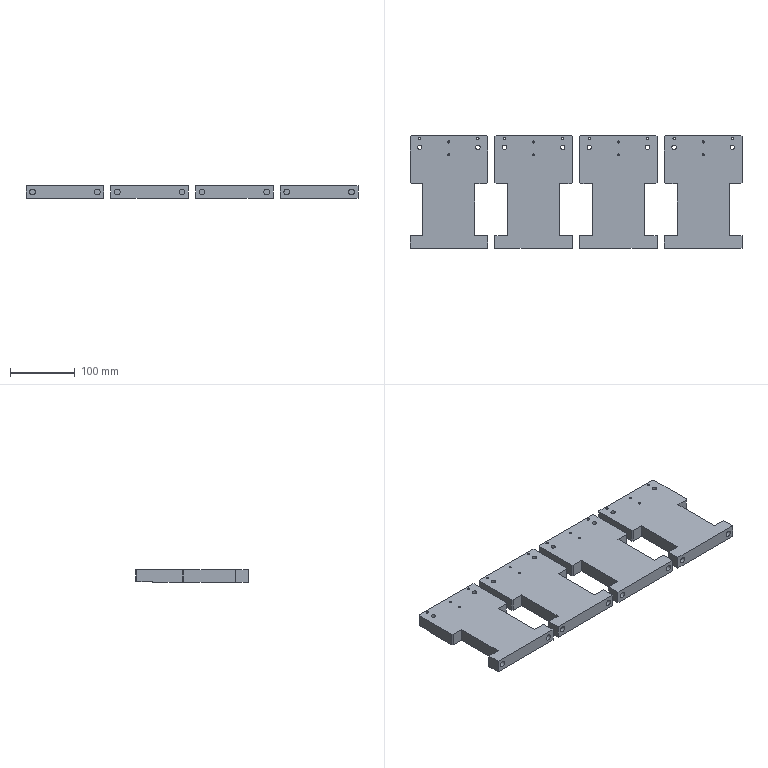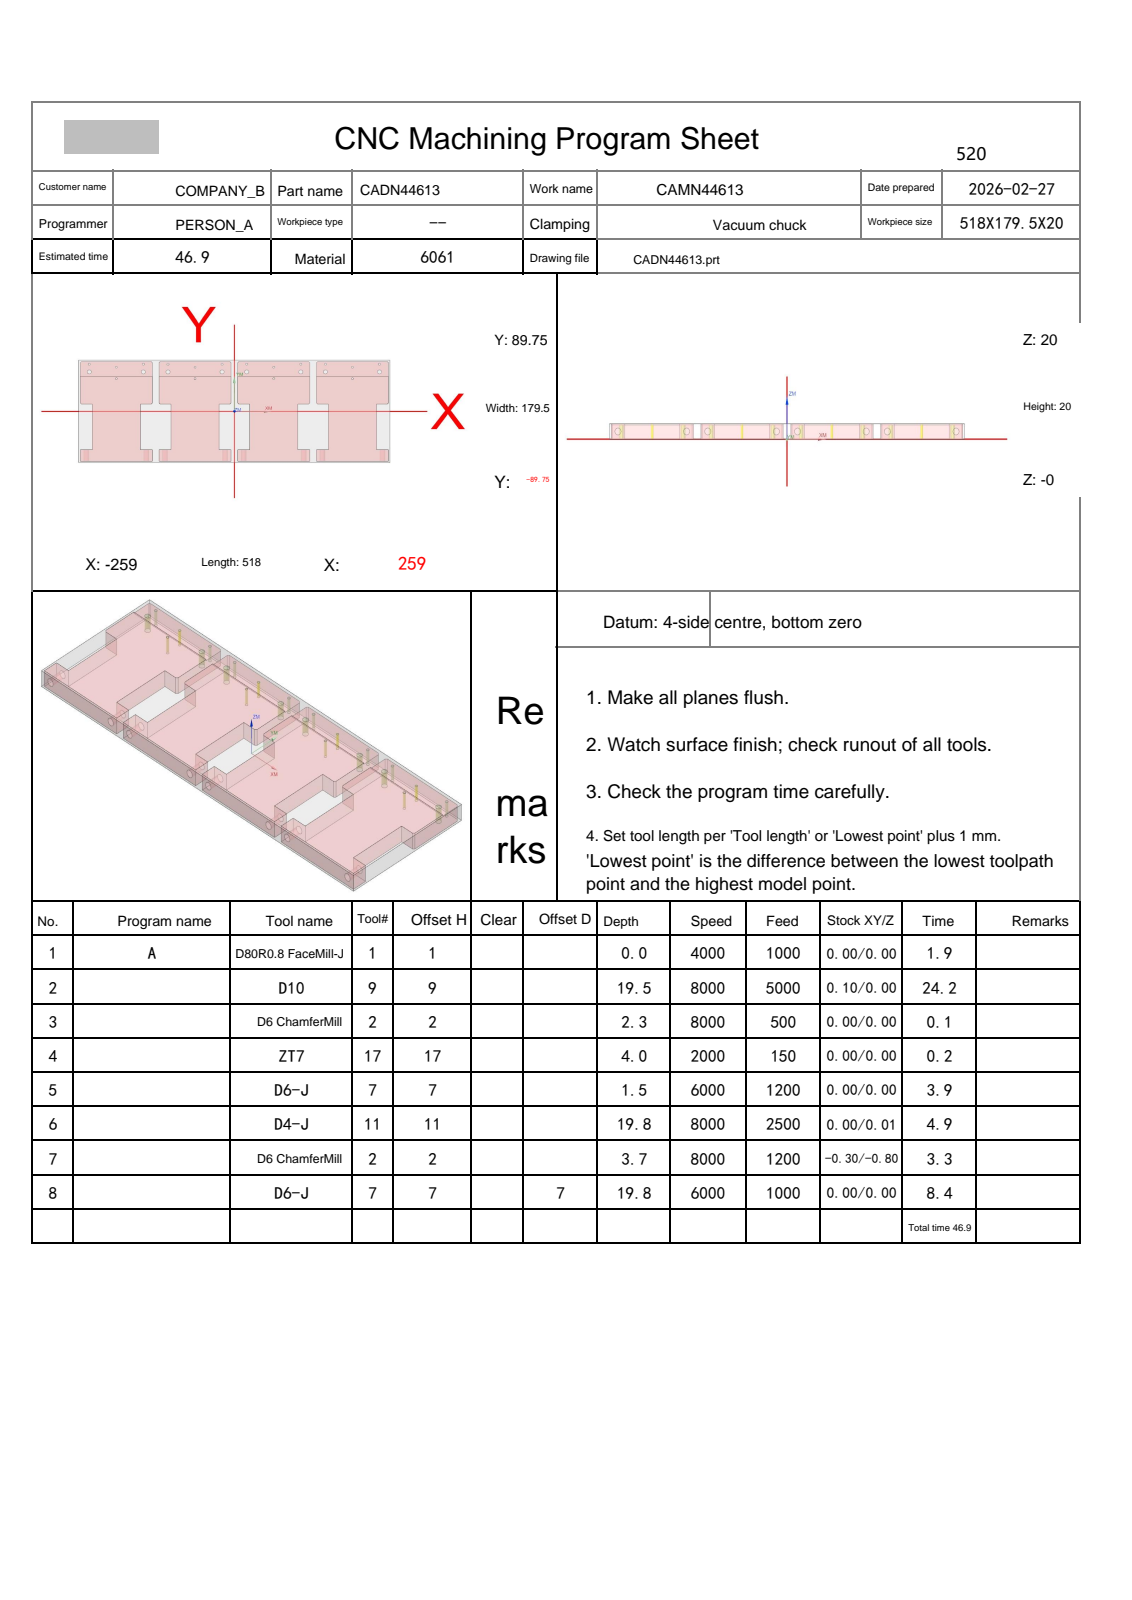NC program | NX | posted by the shop | part box 513 x 174.5 x 20 mm
Lines 5165 to 6116 of 36838:
N6 T11 M06
(D4-J  D=4. R=0. H=11 ce=0.00 di=0.01)
G00 G90 G54 X-242.053 Y-64.649 M03 S8000
G43 H11 Z50.
M08
Z20.3
G01 X-242.052 Y-64.655 Z20.214 F2000.
X-242.049 Y-64.675 Z20.136
X-242.044 Y-64.704 Z20.066
X-242.036 Y-64.743 Z20.004
X-242.025 Y-64.788 Z19.948
X-242.011 Y-64.839 Z19.899
X-241.994 Y-64.893 Z19.857
X-241.973 Y-64.949 Z19.82
X-241.949 Y-65.005 Z19.789
X-241.92 Y-65.06 Z19.763
X-241.888 Y-65.111 Z19.742
X-241.851 Y-65.156 Z19.726
X-241.809 Y-65.195 Z19.714
X-241.762 Y-65.224 Z19.706
X-241.71 Y-65.243 Z19.701
X-241.653 Y-65.25 Z19.7
X-238.5 F2500.
Y-62.097
X-238.516 Y-62.054 Z19.699
X-238.562 Y-62.032 Z19.696
X-238.634 Y-62.031 Z19.692
X-238.729 Y-62.048 Z19.687
X-238.844 Y-62.081 Z19.68
X-238.974 Y-62.13 Z19.672
X-239.118 Y-62.193 Z19.662
X-239.27 Y-62.267 Z19.653
X-239.429 Y-62.352 Z19.642
X-239.59 Y-62.446 Z19.631
X-239.75 Y-62.546 Z19.619
X-240.087 Y-62.788 Z19.592
X-240.403 Y-63.055 Z19.564
X-240.694 Y-63.347 Z19.536
X-240.962 Y-63.662 Z19.508
X-241.203 Y-64. Z19.481
X-241.304 Y-64.16 Z19.469
X-241.398 Y-64.321 Z19.458
X-241.483 Y-64.479 Z19.447
X-241.557 Y-64.632 Z19.438
X-241.62 Y-64.775 Z19.428
X-241.669 Y-64.906 Z19.42
X-241.702 Y-65.021 Z19.413
X-241.719 Y-65.116 Z19.408
X-241.718 Y-65.188 Z19.404
X-241.696 Y-65.234 Z19.401
X-241.653 Y-65.25 Z19.4
X-238.5
Y-62.097
X-238.516 Y-62.054 Z19.399
X-238.562 Y-62.032 Z19.396
X-238.634 Y-62.031 Z19.392
X-238.729 Y-62.048 Z19.387
X-238.844 Y-62.081 Z19.38
X-238.974 Y-62.13 Z19.372
X-239.118 Y-62.193 Z19.362
X-239.27 Y-62.267 Z19.353
X-239.429 Y-62.352 Z19.342
X-239.59 Y-62.446 Z19.331
X-239.75 Y-62.546 Z19.319
X-240.087 Y-62.788 Z19.292
X-240.403 Y-63.055 Z19.264
X-240.694 Y-63.347 Z19.236
X-240.962 Y-63.662 Z19.208
X-241.203 Y-64. Z19.181
X-241.304 Y-64.16 Z19.169
X-241.398 Y-64.321 Z19.158
X-241.483 Y-64.479 Z19.147
X-241.557 Y-64.632 Z19.138
X-241.62 Y-64.775 Z19.128
X-241.669 Y-64.906 Z19.12
X-241.702 Y-65.021 Z19.113
X-241.719 Y-65.116 Z19.108
X-241.718 Y-65.188 Z19.104
X-241.696 Y-65.234 Z19.101
X-241.653 Y-65.25 Z19.1
X-238.5
Y-62.097
X-238.516 Y-62.054 Z19.099
X-238.562 Y-62.032 Z19.096
X-238.634 Y-62.031 Z19.092
X-238.729 Y-62.048 Z19.087
X-238.844 Y-62.081 Z19.08
X-238.974 Y-62.13 Z19.072
X-239.118 Y-62.193 Z19.062
X-239.27 Y-62.267 Z19.053
X-239.429 Y-62.352 Z19.042
X-239.59 Y-62.446 Z19.031
X-239.75 Y-62.546 Z19.019
X-240.087 Y-62.788 Z18.992
X-240.403 Y-63.055 Z18.964
X-240.694 Y-63.347 Z18.936
X-240.962 Y-63.662 Z18.908
X-241.203 Y-64. Z18.881
X-241.304 Y-64.16 Z18.869
X-241.398 Y-64.321 Z18.858
X-241.483 Y-64.479 Z18.847
X-241.557 Y-64.632 Z18.838
X-241.62 Y-64.775 Z18.828
X-241.669 Y-64.906 Z18.82
X-241.702 Y-65.021 Z18.813
X-241.719 Y-65.116 Z18.808
X-241.718 Y-65.188 Z18.804
X-241.696 Y-65.234 Z18.801
X-241.653 Y-65.25 Z18.8
X-238.5
Y-62.097
X-238.516 Y-62.054 Z18.799
X-238.562 Y-62.032 Z18.796
X-238.634 Y-62.031 Z18.792
X-238.729 Y-62.048 Z18.787
X-238.844 Y-62.081 Z18.78
X-238.974 Y-62.13 Z18.772
X-239.118 Y-62.193 Z18.762
X-239.27 Y-62.267 Z18.753
X-239.429 Y-62.352 Z18.742
X-239.59 Y-62.446 Z18.731
X-239.75 Y-62.546 Z18.719
X-240.087 Y-62.788 Z18.692
X-240.403 Y-63.055 Z18.664
X-240.694 Y-63.347 Z18.636
X-240.962 Y-63.662 Z18.608
X-241.203 Y-64. Z18.581
X-241.304 Y-64.16 Z18.569
X-241.398 Y-64.321 Z18.558
X-241.483 Y-64.479 Z18.547
X-241.557 Y-64.632 Z18.538
X-241.62 Y-64.775 Z18.528
X-241.669 Y-64.906 Z18.52
X-241.702 Y-65.021 Z18.513
X-241.719 Y-65.116 Z18.508
X-241.718 Y-65.188 Z18.504
X-241.696 Y-65.234 Z18.501
X-241.653 Y-65.25 Z18.5
X-238.5
Y-62.097
X-238.516 Y-62.054 Z18.499
X-238.562 Y-62.032 Z18.496
X-238.634 Y-62.031 Z18.492
X-238.729 Y-62.048 Z18.487
X-238.844 Y-62.081 Z18.48
X-238.974 Y-62.13 Z18.472
X-239.118 Y-62.193 Z18.462
X-239.27 Y-62.267 Z18.453
X-239.429 Y-62.352 Z18.442
X-239.59 Y-62.446 Z18.431
X-239.75 Y-62.546 Z18.419
X-240.087 Y-62.788 Z18.392
X-240.403 Y-63.055 Z18.364
X-240.694 Y-63.347 Z18.336
X-240.962 Y-63.662 Z18.308
X-241.203 Y-64. Z18.281
X-241.304 Y-64.16 Z18.269
X-241.398 Y-64.321 Z18.258
X-241.483 Y-64.479 Z18.247
X-241.557 Y-64.632 Z18.238
X-241.62 Y-64.775 Z18.228
X-241.669 Y-64.906 Z18.22
X-241.702 Y-65.021 Z18.213
X-241.719 Y-65.116 Z18.208
X-241.718 Y-65.188 Z18.204
X-241.696 Y-65.234 Z18.201
X-241.653 Y-65.25 Z18.2
X-238.5
Y-62.097
X-238.516 Y-62.054 Z18.199
X-238.562 Y-62.032 Z18.196
X-238.634 Y-62.031 Z18.192
X-238.729 Y-62.048 Z18.187
X-238.844 Y-62.081 Z18.18
X-238.974 Y-62.13 Z18.172
X-239.118 Y-62.193 Z18.162
X-239.27 Y-62.267 Z18.153
X-239.429 Y-62.352 Z18.142
X-239.59 Y-62.446 Z18.131
X-239.75 Y-62.546 Z18.119
X-240.087 Y-62.788 Z18.092
X-240.403 Y-63.055 Z18.064
X-240.694 Y-63.347 Z18.036
X-240.962 Y-63.662 Z18.008
X-241.203 Y-64. Z17.981
X-241.304 Y-64.16 Z17.969
X-241.398 Y-64.321 Z17.958
X-241.483 Y-64.479 Z17.947
X-241.557 Y-64.632 Z17.938
X-241.62 Y-64.775 Z17.928
X-241.669 Y-64.906 Z17.92
X-241.702 Y-65.021 Z17.913
X-241.719 Y-65.116 Z17.908
X-241.718 Y-65.188 Z17.904
X-241.696 Y-65.234 Z17.901
X-241.653 Y-65.25 Z17.9
X-238.5
Y-62.097
X-238.516 Y-62.054 Z17.899
X-238.562 Y-62.032 Z17.896
X-238.634 Y-62.031 Z17.892
X-238.729 Y-62.048 Z17.887
X-238.844 Y-62.081 Z17.88
X-238.974 Y-62.13 Z17.872
X-239.118 Y-62.193 Z17.862
X-239.27 Y-62.267 Z17.853
X-239.429 Y-62.352 Z17.842
X-239.59 Y-62.446 Z17.831
X-239.75 Y-62.546 Z17.819
X-240.087 Y-62.788 Z17.792
X-240.403 Y-63.055 Z17.764
X-240.694 Y-63.347 Z17.736
X-240.962 Y-63.662 Z17.708
X-241.203 Y-64. Z17.681
X-241.304 Y-64.16 Z17.669
X-241.398 Y-64.321 Z17.658
X-241.483 Y-64.479 Z17.647
X-241.557 Y-64.632 Z17.638
X-241.62 Y-64.775 Z17.628
X-241.669 Y-64.906 Z17.62
X-241.702 Y-65.021 Z17.613
X-241.719 Y-65.116 Z17.608
X-241.718 Y-65.188 Z17.604
X-241.696 Y-65.234 Z17.601
X-241.653 Y-65.25 Z17.6
X-238.5
Y-62.097
X-238.516 Y-62.054 Z17.599
X-238.562 Y-62.032 Z17.596
X-238.634 Y-62.031 Z17.592
X-238.729 Y-62.048 Z17.587
X-238.844 Y-62.081 Z17.58
X-238.974 Y-62.13 Z17.572
X-239.118 Y-62.193 Z17.562
X-239.27 Y-62.267 Z17.553
X-239.429 Y-62.352 Z17.542
X-239.59 Y-62.446 Z17.531
X-239.75 Y-62.546 Z17.519
X-240.087 Y-62.788 Z17.492
X-240.403 Y-63.055 Z17.464
X-240.694 Y-63.347 Z17.436
X-240.962 Y-63.662 Z17.408
X-241.203 Y-64. Z17.381
X-241.304 Y-64.16 Z17.369
X-241.398 Y-64.321 Z17.358
X-241.483 Y-64.479 Z17.347
X-241.557 Y-64.632 Z17.338
X-241.62 Y-64.775 Z17.328
X-241.669 Y-64.906 Z17.32
X-241.702 Y-65.021 Z17.313
X-241.719 Y-65.116 Z17.308
X-241.718 Y-65.188 Z17.304
X-241.696 Y-65.234 Z17.301
X-241.653 Y-65.25 Z17.3
X-238.5
Y-62.097
X-238.516 Y-62.054 Z17.299
X-238.562 Y-62.032 Z17.296
X-238.634 Y-62.031 Z17.292
X-238.729 Y-62.048 Z17.287
X-238.844 Y-62.081 Z17.28
X-238.974 Y-62.13 Z17.272
X-239.118 Y-62.193 Z17.262
X-239.27 Y-62.267 Z17.253
X-239.429 Y-62.352 Z17.242
X-239.59 Y-62.446 Z17.231
X-239.75 Y-62.546 Z17.219
X-240.087 Y-62.788 Z17.192
X-240.403 Y-63.055 Z17.164
X-240.694 Y-63.347 Z17.136
X-240.962 Y-63.662 Z17.108
X-241.203 Y-64. Z17.081
X-241.304 Y-64.16 Z17.069
X-241.398 Y-64.321 Z17.058
X-241.483 Y-64.479 Z17.047
X-241.557 Y-64.632 Z17.038
X-241.62 Y-64.775 Z17.028
X-241.669 Y-64.906 Z17.02
X-241.702 Y-65.021 Z17.013
X-241.719 Y-65.116 Z17.008
X-241.718 Y-65.188 Z17.004
X-241.696 Y-65.234 Z17.001
X-241.653 Y-65.25 Z17.
X-238.5
Y-62.097
X-238.516 Y-62.054 Z16.999
X-238.562 Y-62.032 Z16.996
X-238.634 Y-62.031 Z16.992
X-238.729 Y-62.048 Z16.987
X-238.844 Y-62.081 Z16.98
X-238.974 Y-62.13 Z16.972
X-239.118 Y-62.193 Z16.962
X-239.27 Y-62.267 Z16.953
X-239.429 Y-62.352 Z16.942
X-239.59 Y-62.446 Z16.931
X-239.75 Y-62.546 Z16.919
X-240.087 Y-62.788 Z16.892
X-240.403 Y-63.055 Z16.864
X-240.694 Y-63.347 Z16.836
X-240.962 Y-63.662 Z16.808
X-241.203 Y-64. Z16.781
X-241.304 Y-64.16 Z16.769
X-241.398 Y-64.321 Z16.758
X-241.483 Y-64.479 Z16.747
X-241.557 Y-64.632 Z16.738
X-241.62 Y-64.775 Z16.728
X-241.669 Y-64.906 Z16.72
X-241.702 Y-65.021 Z16.713
X-241.719 Y-65.116 Z16.708
X-241.718 Y-65.188 Z16.704
X-241.696 Y-65.234 Z16.701
X-241.653 Y-65.25 Z16.7
X-238.5
Y-62.097
X-238.516 Y-62.054 Z16.699
X-238.562 Y-62.032 Z16.696
X-238.634 Y-62.031 Z16.692
X-238.729 Y-62.048 Z16.687
X-238.844 Y-62.081 Z16.68
X-238.974 Y-62.13 Z16.672
X-239.118 Y-62.193 Z16.662
X-239.27 Y-62.267 Z16.653
X-239.429 Y-62.352 Z16.642
X-239.59 Y-62.446 Z16.631
X-239.75 Y-62.546 Z16.619
X-240.087 Y-62.788 Z16.592
X-240.403 Y-63.055 Z16.564
X-240.694 Y-63.347 Z16.536
X-240.962 Y-63.662 Z16.508
X-241.203 Y-64. Z16.481
X-241.304 Y-64.16 Z16.469
X-241.398 Y-64.321 Z16.458
X-241.483 Y-64.479 Z16.447
X-241.557 Y-64.632 Z16.438
X-241.62 Y-64.775 Z16.428
X-241.669 Y-64.906 Z16.42
X-241.702 Y-65.021 Z16.413
X-241.719 Y-65.116 Z16.408
X-241.718 Y-65.188 Z16.404
X-241.696 Y-65.234 Z16.401
X-241.653 Y-65.25 Z16.4
X-238.5
Y-62.097
X-238.516 Y-62.054 Z16.399
X-238.562 Y-62.032 Z16.396
X-238.634 Y-62.031 Z16.392
X-238.729 Y-62.048 Z16.387
X-238.844 Y-62.081 Z16.38
X-238.974 Y-62.13 Z16.372
X-239.118 Y-62.193 Z16.362
X-239.27 Y-62.267 Z16.353
X-239.429 Y-62.352 Z16.342
X-239.59 Y-62.446 Z16.331
X-239.75 Y-62.546 Z16.319
X-240.087 Y-62.788 Z16.292
X-240.403 Y-63.055 Z16.264
X-240.694 Y-63.347 Z16.236
X-240.962 Y-63.662 Z16.208
X-241.203 Y-64. Z16.181
X-241.304 Y-64.16 Z16.169
X-241.398 Y-64.321 Z16.158
X-241.483 Y-64.479 Z16.147
X-241.557 Y-64.632 Z16.138
X-241.62 Y-64.775 Z16.128
X-241.669 Y-64.906 Z16.12
X-241.702 Y-65.021 Z16.113
X-241.719 Y-65.116 Z16.108
X-241.718 Y-65.188 Z16.104
X-241.696 Y-65.234 Z16.101
X-241.653 Y-65.25 Z16.1
X-238.5
Y-62.097
X-238.516 Y-62.054 Z16.099
X-238.562 Y-62.032 Z16.096
X-238.634 Y-62.031 Z16.092
X-238.729 Y-62.048 Z16.087
X-238.844 Y-62.081 Z16.08
X-238.974 Y-62.13 Z16.072
X-239.118 Y-62.193 Z16.062
X-239.27 Y-62.267 Z16.053
X-239.429 Y-62.352 Z16.042
X-239.59 Y-62.446 Z16.031
X-239.75 Y-62.546 Z16.019
X-240.087 Y-62.788 Z15.992
X-240.403 Y-63.055 Z15.964
X-240.694 Y-63.347 Z15.936
X-240.962 Y-63.662 Z15.908
X-241.203 Y-64. Z15.881
X-241.304 Y-64.16 Z15.869
X-241.398 Y-64.321 Z15.858
X-241.483 Y-64.479 Z15.847
X-241.557 Y-64.632 Z15.838
X-241.62 Y-64.775 Z15.828
X-241.669 Y-64.906 Z15.82
X-241.702 Y-65.021 Z15.813
X-241.719 Y-65.116 Z15.808
X-241.718 Y-65.188 Z15.804
X-241.696 Y-65.234 Z15.801
X-241.653 Y-65.25 Z15.8
X-238.5
Y-62.097
X-238.516 Y-62.054 Z15.799
X-238.562 Y-62.032 Z15.796
X-238.634 Y-62.031 Z15.792
X-238.729 Y-62.048 Z15.787
X-238.844 Y-62.081 Z15.78
X-238.974 Y-62.13 Z15.772
X-239.118 Y-62.193 Z15.762
X-239.27 Y-62.267 Z15.753
X-239.429 Y-62.352 Z15.742
X-239.59 Y-62.446 Z15.731
X-239.75 Y-62.546 Z15.719
X-240.087 Y-62.788 Z15.692
X-240.403 Y-63.055 Z15.664
X-240.694 Y-63.347 Z15.636
X-240.962 Y-63.662 Z15.608
X-241.203 Y-64. Z15.581
X-241.304 Y-64.16 Z15.569
X-241.398 Y-64.321 Z15.558
X-241.483 Y-64.479 Z15.547
X-241.557 Y-64.632 Z15.538
X-241.62 Y-64.775 Z15.528
X-241.669 Y-64.906 Z15.52
X-241.702 Y-65.021 Z15.513
X-241.719 Y-65.116 Z15.508
X-241.718 Y-65.188 Z15.504
X-241.696 Y-65.234 Z15.501
X-241.653 Y-65.25 Z15.5
X-238.5
Y-62.097
X-238.516 Y-62.054 Z15.499
X-238.562 Y-62.032 Z15.496
X-238.634 Y-62.031 Z15.492
X-238.729 Y-62.048 Z15.487
X-238.844 Y-62.081 Z15.48
X-238.974 Y-62.13 Z15.472
X-239.118 Y-62.193 Z15.462
X-239.27 Y-62.267 Z15.453
X-239.429 Y-62.352 Z15.442
X-239.59 Y-62.446 Z15.431
X-239.75 Y-62.546 Z15.419
X-240.087 Y-62.788 Z15.392
X-240.403 Y-63.055 Z15.364
X-240.694 Y-63.347 Z15.336
X-240.962 Y-63.662 Z15.308
X-241.203 Y-64. Z15.281
X-241.304 Y-64.16 Z15.269
X-241.398 Y-64.321 Z15.258
X-241.483 Y-64.479 Z15.247
X-241.557 Y-64.632 Z15.238
X-241.62 Y-64.775 Z15.228
X-241.669 Y-64.906 Z15.22
X-241.702 Y-65.021 Z15.213
X-241.719 Y-65.116 Z15.208
X-241.718 Y-65.188 Z15.204
X-241.696 Y-65.234 Z15.201
X-241.653 Y-65.25 Z15.2
X-238.5
Y-62.097
X-238.516 Y-62.054 Z15.199
X-238.562 Y-62.032 Z15.196
X-238.634 Y-62.031 Z15.192
X-238.729 Y-62.048 Z15.187
X-238.844 Y-62.081 Z15.18
X-238.974 Y-62.13 Z15.172
X-239.118 Y-62.193 Z15.162
X-239.27 Y-62.267 Z15.153
X-239.429 Y-62.352 Z15.142
X-239.59 Y-62.446 Z15.131
X-239.75 Y-62.546 Z15.119
X-240.087 Y-62.788 Z15.092
X-240.403 Y-63.055 Z15.064
X-240.694 Y-63.347 Z15.036
X-240.962 Y-63.662 Z15.008
X-241.203 Y-64. Z14.981
X-241.304 Y-64.16 Z14.969
X-241.398 Y-64.321 Z14.958
X-241.483 Y-64.479 Z14.947
X-241.557 Y-64.632 Z14.938
X-241.62 Y-64.775 Z14.928
X-241.669 Y-64.906 Z14.92
X-241.702 Y-65.021 Z14.913
X-241.719 Y-65.116 Z14.908
X-241.718 Y-65.188 Z14.904
X-241.696 Y-65.234 Z14.901
X-241.653 Y-65.25 Z14.9
X-238.5
Y-62.097
X-238.516 Y-62.054 Z14.899
X-238.562 Y-62.032 Z14.896
X-238.634 Y-62.031 Z14.892
X-238.729 Y-62.048 Z14.887
X-238.844 Y-62.081 Z14.88
X-238.974 Y-62.13 Z14.872
X-239.118 Y-62.193 Z14.862
X-239.27 Y-62.267 Z14.853
X-239.429 Y-62.352 Z14.842
X-239.59 Y-62.446 Z14.831
X-239.75 Y-62.546 Z14.819
X-240.087 Y-62.788 Z14.792
X-240.403 Y-63.055 Z14.764
X-240.694 Y-63.347 Z14.736
X-240.962 Y-63.662 Z14.708
X-241.203 Y-64. Z14.681
X-241.304 Y-64.16 Z14.669
X-241.398 Y-64.321 Z14.658
X-241.483 Y-64.479 Z14.647
X-241.557 Y-64.632 Z14.638
X-241.62 Y-64.775 Z14.628
X-241.669 Y-64.906 Z14.62
X-241.702 Y-65.021 Z14.613
X-241.719 Y-65.116 Z14.608
X-241.718 Y-65.188 Z14.604
X-241.696 Y-65.234 Z14.601
X-241.653 Y-65.25 Z14.6
X-238.5
Y-62.097
X-238.516 Y-62.054 Z14.599
X-238.562 Y-62.032 Z14.596
X-238.634 Y-62.031 Z14.592
X-238.729 Y-62.048 Z14.587
X-238.844 Y-62.081 Z14.58
X-238.974 Y-62.13 Z14.572
X-239.118 Y-62.193 Z14.562
X-239.27 Y-62.267 Z14.553
X-239.429 Y-62.352 Z14.542
X-239.59 Y-62.446 Z14.531
X-239.75 Y-62.546 Z14.519
X-240.087 Y-62.788 Z14.492
X-240.403 Y-63.055 Z14.464
X-240.694 Y-63.347 Z14.436
X-240.962 Y-63.662 Z14.408
X-241.203 Y-64. Z14.381
X-241.304 Y-64.16 Z14.369
X-241.398 Y-64.321 Z14.358
X-241.483 Y-64.479 Z14.347
X-241.557 Y-64.632 Z14.338
X-241.62 Y-64.775 Z14.328
X-241.669 Y-64.906 Z14.32
X-241.702 Y-65.021 Z14.313
X-241.719 Y-65.116 Z14.308
X-241.718 Y-65.188 Z14.304
X-241.696 Y-65.234 Z14.301
X-241.653 Y-65.25 Z14.3
X-238.5
Y-62.097
X-238.516 Y-62.054 Z14.299
X-238.562 Y-62.032 Z14.296
X-238.634 Y-62.031 Z14.292
X-238.729 Y-62.048 Z14.287
X-238.844 Y-62.081 Z14.28
X-238.974 Y-62.13 Z14.272
X-239.118 Y-62.193 Z14.262
X-239.27 Y-62.267 Z14.253
X-239.429 Y-62.352 Z14.242
X-239.59 Y-62.446 Z14.231
X-239.75 Y-62.546 Z14.219
X-240.087 Y-62.788 Z14.192
X-240.403 Y-63.055 Z14.164
X-240.694 Y-63.347 Z14.136
X-240.962 Y-63.662 Z14.108
X-241.203 Y-64. Z14.081
X-241.304 Y-64.16 Z14.069
X-241.398 Y-64.321 Z14.058
X-241.483 Y-64.479 Z14.047
X-241.557 Y-64.632 Z14.038
X-241.62 Y-64.775 Z14.028
X-241.669 Y-64.906 Z14.02
X-241.702 Y-65.021 Z14.013
X-241.719 Y-65.116 Z14.008
X-241.718 Y-65.188 Z14.004
X-241.696 Y-65.234 Z14.001
X-241.653 Y-65.25 Z14.
X-238.5
Y-62.097
X-238.516 Y-62.054 Z13.999
X-238.562 Y-62.032 Z13.996
X-238.634 Y-62.031 Z13.992
X-238.729 Y-62.048 Z13.987
X-238.844 Y-62.081 Z13.98
X-238.974 Y-62.13 Z13.972
X-239.118 Y-62.193 Z13.962
X-239.27 Y-62.267 Z13.953
X-239.429 Y-62.352 Z13.942
X-239.59 Y-62.446 Z13.931
X-239.75 Y-62.546 Z13.919
X-240.087 Y-62.788 Z13.892
X-240.403 Y-63.055 Z13.864
X-240.694 Y-63.347 Z13.836
X-240.962 Y-63.662 Z13.808
X-241.203 Y-64. Z13.781
X-241.304 Y-64.16 Z13.769
X-241.398 Y-64.321 Z13.758
X-241.483 Y-64.479 Z13.747
X-241.557 Y-64.632 Z13.738
X-241.62 Y-64.775 Z13.728
X-241.669 Y-64.906 Z13.72
X-241.702 Y-65.021 Z13.713
X-241.719 Y-65.116 Z13.708
X-241.718 Y-65.188 Z13.704
X-241.696 Y-65.234 Z13.701
X-241.653 Y-65.25 Z13.7
X-238.5
Y-62.097
X-238.516 Y-62.054 Z13.699
X-238.562 Y-62.032 Z13.696
X-238.634 Y-62.031 Z13.692
X-238.729 Y-62.048 Z13.687
X-238.844 Y-62.081 Z13.68
X-238.974 Y-62.13 Z13.672
X-239.118 Y-62.193 Z13.662
X-239.27 Y-62.267 Z13.653
X-239.429 Y-62.352 Z13.642
X-239.59 Y-62.446 Z13.631
X-239.75 Y-62.546 Z13.619
X-240.087 Y-62.788 Z13.592
X-240.403 Y-63.055 Z13.564
X-240.694 Y-63.347 Z13.536
X-240.962 Y-63.662 Z13.508
X-241.203 Y-64. Z13.481
X-241.304 Y-64.16 Z13.469
X-241.398 Y-64.321 Z13.458
X-241.483 Y-64.479 Z13.447
X-241.557 Y-64.632 Z13.438
X-241.62 Y-64.775 Z13.428
X-241.669 Y-64.906 Z13.42
X-241.702 Y-65.021 Z13.413
X-241.719 Y-65.116 Z13.408
X-241.718 Y-65.188 Z13.404
X-241.696 Y-65.234 Z13.401
X-241.653 Y-65.25 Z13.4
X-238.5
Y-62.097
X-238.516 Y-62.054 Z13.399
X-238.562 Y-62.032 Z13.396
X-238.634 Y-62.031 Z13.392
X-238.729 Y-62.048 Z13.387
X-238.844 Y-62.081 Z13.38
X-238.974 Y-62.13 Z13.372
X-239.118 Y-62.193 Z13.362
X-239.27 Y-62.267 Z13.353
X-239.429 Y-62.352 Z13.342
X-239.59 Y-62.446 Z13.331
X-239.75 Y-62.546 Z13.319
X-240.087 Y-62.788 Z13.292
X-240.403 Y-63.055 Z13.264
X-240.694 Y-63.347 Z13.236
X-240.962 Y-63.662 Z13.208
X-241.203 Y-64. Z13.181
X-241.304 Y-64.16 Z13.169
X-241.398 Y-64.321 Z13.158
X-241.483 Y-64.479 Z13.147
X-241.557 Y-64.632 Z13.138
X-241.62 Y-64.775 Z13.128
X-241.669 Y-64.906 Z13.12
X-241.702 Y-65.021 Z13.113
X-241.719 Y-65.116 Z13.108
X-241.718 Y-65.188 Z13.104
X-241.696 Y-65.234 Z13.101
X-241.653 Y-65.25 Z13.1
X-238.5
Y-62.097
X-238.516 Y-62.054 Z13.099
X-238.562 Y-62.032 Z13.096
X-238.634 Y-62.031 Z13.092
X-238.729 Y-62.048 Z13.087
X-238.844 Y-62.081 Z13.08
X-238.974 Y-62.13 Z13.072
X-239.118 Y-62.193 Z13.062
X-239.27 Y-62.267 Z13.053
X-239.429 Y-62.352 Z13.042
X-239.59 Y-62.446 Z13.031
X-239.75 Y-62.546 Z13.019
X-240.087 Y-62.788 Z12.992
X-240.403 Y-63.055 Z12.964
X-240.694 Y-63.347 Z12.936
X-240.962 Y-63.662 Z12.908
X-241.203 Y-64. Z12.881
X-241.304 Y-64.16 Z12.869
X-241.398 Y-64.321 Z12.858
X-241.483 Y-64.479 Z12.847
X-241.557 Y-64.632 Z12.838
X-241.62 Y-64.775 Z12.828
X-241.669 Y-64.906 Z12.82
X-241.702 Y-65.021 Z12.813
X-241.719 Y-65.116 Z12.808
X-241.718 Y-65.188 Z12.804
X-241.696 Y-65.234 Z12.801
X-241.653 Y-65.25 Z12.8
X-238.5
Y-62.097
X-238.516 Y-62.054 Z12.799
X-238.562 Y-62.032 Z12.796
X-238.634 Y-62.031 Z12.792
X-238.729 Y-62.048 Z12.787
X-238.844 Y-62.081 Z12.78
X-238.974 Y-62.13 Z12.772
X-239.118 Y-62.193 Z12.762
X-239.27 Y-62.267 Z12.753
X-239.429 Y-62.352 Z12.742
X-239.59 Y-62.446 Z12.731
X-239.75 Y-62.546 Z12.719
X-240.087 Y-62.788 Z12.692
X-240.403 Y-63.055 Z12.664
X-240.694 Y-63.347 Z12.636
X-240.962 Y-63.662 Z12.608
X-241.203 Y-64. Z12.581
X-241.304 Y-64.16 Z12.569
X-241.398 Y-64.321 Z12.558
X-241.483 Y-64.479 Z12.547
X-241.557 Y-64.632 Z12.538
X-241.62 Y-64.775 Z12.528
X-241.669 Y-64.906 Z12.52
X-241.702 Y-65.021 Z12.513
X-241.719 Y-65.116 Z12.508
X-241.718 Y-65.188 Z12.504
X-241.696 Y-65.234 Z12.501
X-241.653 Y-65.25 Z12.5
X-238.5
Y-62.097
X-238.516 Y-62.054 Z12.499
X-238.562 Y-62.032 Z12.496
X-238.634 Y-62.031 Z12.492
X-238.729 Y-62.048 Z12.487
X-238.844 Y-62.081 Z12.48
X-238.974 Y-62.13 Z12.472
X-239.118 Y-62.193 Z12.462
X-239.27 Y-62.267 Z12.453
X-239.429 Y-62.352 Z12.442
X-239.59 Y-62.446 Z12.431
X-239.75 Y-62.546 Z12.419
X-240.087 Y-62.788 Z12.392
X-240.403 Y-63.055 Z12.364
X-240.694 Y-63.347 Z12.336
X-240.962 Y-63.662 Z12.308
X-241.203 Y-64. Z12.281
X-241.304 Y-64.16 Z12.269
X-241.398 Y-64.321 Z12.258
X-241.483 Y-64.479 Z12.247
X-241.557 Y-64.632 Z12.238
X-241.62 Y-64.775 Z12.228
X-241.669 Y-64.906 Z12.22
X-241.702 Y-65.021 Z12.213
X-241.719 Y-65.116 Z12.208
X-241.718 Y-65.188 Z12.204
X-241.696 Y-65.234 Z12.201
X-241.653 Y-65.25 Z12.2
X-238.5
Y-62.097
X-238.516 Y-62.054 Z12.199
X-238.562 Y-62.032 Z12.196
X-238.634 Y-62.031 Z12.192
X-238.729 Y-62.048 Z12.187
X-238.844 Y-62.081 Z12.18
X-238.974 Y-62.13 Z12.172
X-239.118 Y-62.193 Z12.162
X-239.27 Y-62.267 Z12.153
X-239.429 Y-62.352 Z12.142
X-239.59 Y-62.446 Z12.131
X-239.75 Y-62.546 Z12.119
X-240.087 Y-62.788 Z12.092
X-240.403 Y-63.055 Z12.064
X-240.694 Y-63.347 Z12.036
X-240.962 Y-63.662 Z12.008
X-241.203 Y-64. Z11.981
X-241.304 Y-64.16 Z11.969
X-241.398 Y-64.321 Z11.958
X-241.483 Y-64.479 Z11.947
X-241.557 Y-64.632 Z11.938
X-241.62 Y-64.775 Z11.928
X-241.669 Y-64.906 Z11.92
X-241.702 Y-65.021 Z11.913
X-241.719 Y-65.116 Z11.908
X-241.718 Y-65.188 Z11.904
X-241.696 Y-65.234 Z11.901
X-241.653 Y-65.25 Z11.9
X-238.5
Y-62.097
X-238.516 Y-62.054 Z11.899
X-238.562 Y-62.032 Z11.896
X-238.634 Y-62.031 Z11.892
X-238.729 Y-62.048 Z11.887
X-238.844 Y-62.081 Z11.88
X-238.974 Y-62.13 Z11.872
X-239.118 Y-62.193 Z11.862
X-239.27 Y-62.267 Z11.853
X-239.429 Y-62.352 Z11.842
X-239.59 Y-62.446 Z11.831
X-239.75 Y-62.546 Z11.819
X-240.087 Y-62.788 Z11.792
X-240.403 Y-63.055 Z11.764
X-240.694 Y-63.347 Z11.736
X-240.962 Y-63.662 Z11.708
X-241.203 Y-64. Z11.681
X-241.304 Y-64.16 Z11.669
X-241.398 Y-64.321 Z11.658
X-241.483 Y-64.479 Z11.647
X-241.557 Y-64.632 Z11.638
X-241.62 Y-64.775 Z11.628
X-241.669 Y-64.906 Z11.62
X-241.702 Y-65.021 Z11.613
X-241.719 Y-65.116 Z11.608
X-241.718 Y-65.188 Z11.604
X-241.696 Y-65.234 Z11.601
X-241.653 Y-65.25 Z11.6
X-238.5
Y-62.097
X-238.516 Y-62.054 Z11.599
X-238.562 Y-62.032 Z11.596
X-238.634 Y-62.031 Z11.592
X-238.729 Y-62.048 Z11.587
X-238.844 Y-62.081 Z11.58
X-238.974 Y-62.13 Z11.572
X-239.118 Y-62.193 Z11.562
X-239.27 Y-62.267 Z11.553
X-239.429 Y-62.352 Z11.542
X-239.59 Y-62.446 Z11.531
X-239.75 Y-62.546 Z11.519
X-240.087 Y-62.788 Z11.492
X-240.403 Y-63.055 Z11.464
X-240.694 Y-63.347 Z11.436
X-240.962 Y-63.662 Z11.408
X-241.203 Y-64. Z11.381
X-241.304 Y-64.16 Z11.369
X-241.398 Y-64.321 Z11.358
X-241.483 Y-64.479 Z11.347
X-241.557 Y-64.632 Z11.338
X-241.62 Y-64.775 Z11.328
X-241.669 Y-64.906 Z11.32
X-241.702 Y-65.021 Z11.313
X-241.719 Y-65.116 Z11.308
X-241.718 Y-65.188 Z11.304
X-241.696 Y-65.234 Z11.301
X-241.653 Y-65.25 Z11.3
X-238.5
Y-62.097
X-238.516 Y-62.054 Z11.299
X-238.562 Y-62.032 Z11.296
X-238.634 Y-62.031 Z11.292
X-238.729 Y-62.048 Z11.287
X-238.844 Y-62.081 Z11.28
X-238.974 Y-62.13 Z11.272
X-239.118 Y-62.193 Z11.262
X-239.27 Y-62.267 Z11.253
X-239.429 Y-62.352 Z11.242
X-239.59 Y-62.446 Z11.231
X-239.75 Y-62.546 Z11.219
X-240.087 Y-62.788 Z11.192
X-240.403 Y-63.055 Z11.164
X-240.694 Y-63.347 Z11.136
X-240.962 Y-63.662 Z11.108
X-241.203 Y-64. Z11.081
X-241.304 Y-64.16 Z11.069
X-241.398 Y-64.321 Z11.058
X-241.483 Y-64.479 Z11.047
X-241.557 Y-64.632 Z11.038
X-241.62 Y-64.775 Z11.028
X-241.669 Y-64.906 Z11.02
X-241.702 Y-65.021 Z11.013
X-241.719 Y-65.116 Z11.008
X-241.718 Y-65.188 Z11.004
X-241.696 Y-65.234 Z11.001
X-241.653 Y-65.25 Z11.
X-238.5
Y-62.097
X-238.516 Y-62.054 Z10.999
X-238.562 Y-62.032 Z10.996
X-238.634 Y-62.031 Z10.992
X-238.729 Y-62.048 Z10.987
X-238.844 Y-62.081 Z10.98
X-238.974 Y-62.13 Z10.972
X-239.118 Y-62.193 Z10.962
X-239.27 Y-62.267 Z10.953
X-239.429 Y-62.352 Z10.942
X-239.59 Y-62.446 Z10.931
X-239.75 Y-62.546 Z10.919
X-240.087 Y-62.788 Z10.892
X-240.403 Y-63.055 Z10.864
X-240.694 Y-63.347 Z10.836
X-240.962 Y-63.662 Z10.808
X-241.203 Y-64. Z10.781
X-241.304 Y-64.16 Z10.769
X-241.398 Y-64.321 Z10.758
X-241.483 Y-64.479 Z10.747
X-241.557 Y-64.632 Z10.738
X-241.62 Y-64.775 Z10.728
X-241.669 Y-64.906 Z10.72
X-241.702 Y-65.021 Z10.713
X-241.719 Y-65.116 Z10.708
X-241.718 Y-65.188 Z10.704
X-241.696 Y-65.234 Z10.701
X-241.653 Y-65.25 Z10.7
X-238.5
Y-62.097
X-238.516 Y-62.054 Z10.699
X-238.562 Y-62.032 Z10.696
X-238.634 Y-62.031 Z10.692
X-238.729 Y-62.048 Z10.687
X-238.844 Y-62.081 Z10.68
X-238.974 Y-62.13 Z10.672
X-239.118 Y-62.193 Z10.662
X-239.27 Y-62.267 Z10.653
X-239.429 Y-62.352 Z10.642
X-239.59 Y-62.446 Z10.631
X-239.75 Y-62.546 Z10.619
X-240.087 Y-62.788 Z10.592
X-240.403 Y-63.055 Z10.564
X-240.694 Y-63.347 Z10.536
X-240.962 Y-63.662 Z10.508
X-241.203 Y-64. Z10.481
X-241.304 Y-64.16 Z10.469
X-241.398 Y-64.321 Z10.458
X-241.483 Y-64.479 Z10.447
X-241.557 Y-64.632 Z10.438
X-241.62 Y-64.775 Z10.428
X-241.669 Y-64.906 Z10.42
X-241.702 Y-65.021 Z10.413
X-241.719 Y-65.116 Z10.408
X-241.718 Y-65.188 Z10.404
X-241.696 Y-65.234 Z10.401
X-241.653 Y-65.25 Z10.4
X-238.5
Y-62.097
X-238.516 Y-62.054 Z10.399
X-238.562 Y-62.032 Z10.396
X-238.634 Y-62.031 Z10.392
X-238.729 Y-62.048 Z10.387
X-238.844 Y-62.081 Z10.38
X-238.974 Y-62.13 Z10.372
X-239.118 Y-62.193 Z10.362
X-239.27 Y-62.267 Z10.353
X-239.429 Y-62.352 Z10.342
X-239.59 Y-62.446 Z10.331
X-239.75 Y-62.546 Z10.319
X-240.087 Y-62.788 Z10.292
X-240.403 Y-63.055 Z10.264
X-240.694 Y-63.347 Z10.236
X-240.962 Y-63.662 Z10.208
X-241.203 Y-64. Z10.181
X-241.304 Y-64.16 Z10.169
X-241.398 Y-64.321 Z10.158
X-241.483 Y-64.479 Z10.147
X-241.557 Y-64.632 Z10.138
X-241.62 Y-64.775 Z10.128
X-241.669 Y-64.906 Z10.12
X-241.702 Y-65.021 Z10.113
X-241.719 Y-65.116 Z10.108
X-241.718 Y-65.188 Z10.104
X-241.696 Y-65.234 Z10.101
X-241.653 Y-65.25 Z10.1
X-238.5
Y-62.097